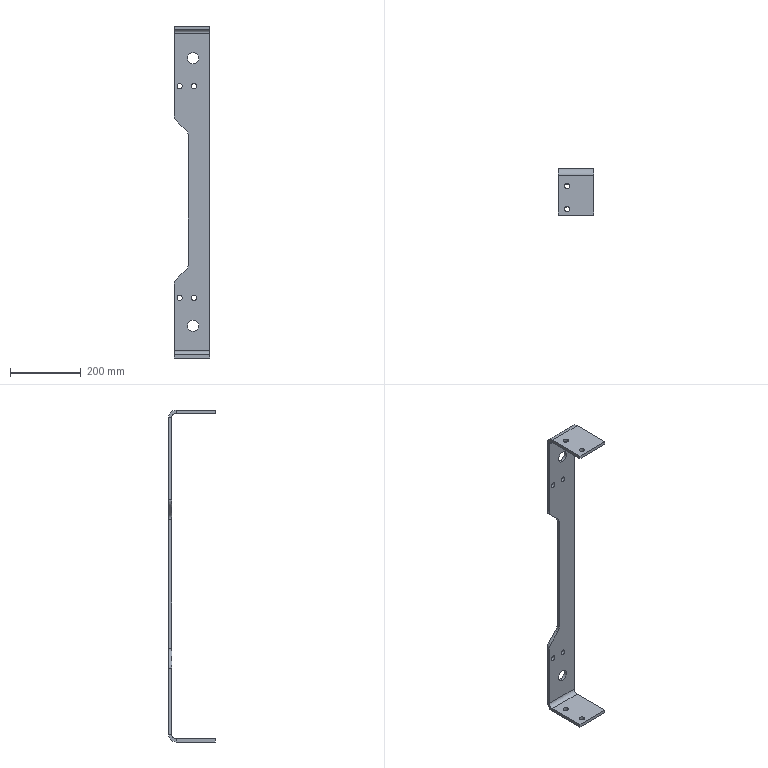Part | SolidWorks | features ICE 2, Fillet 1, FlatPattern 1, SMBaseFlange 1, SheetMetal 1 | 1 solid | 50 faces | box 100 x 132 x 940 mm | volume 876071 mm3 | cylinder 28 | plane 22 | commonest cylinder face diameters 15 x16 32.2 x4 40 x4 24 x2 42 x2
STEP:
#1=CARTESIAN_POINT('',(32.5,17.,-931.));
#2=VERTEX_POINT('',#1);
#3=CARTESIAN_POINT('',(17.5,17.,-931.));
#4=VERTEX_POINT('',#3);
#5=CARTESIAN_POINT('',(25.,17.,-931.));
#6=DIRECTION('',(0.,0.,-1.));
#7=DIRECTION('',(-1.,0.,0.));
#8=AXIS2_PLACEMENT_3D('',#5,#6,#7);
#9=CIRCLE('',#8,7.5);
#10=EDGE_CURVE('',#2,#4,#9,.T.);
#11=ORIENTED_EDGE('',*,*,#10,.F.);
#12=CARTESIAN_POINT('',(32.5,17.,-940.));
#13=VERTEX_POINT('',#12);
#14=CARTESIAN_POINT('',(32.5,17.,0.));
#15=DIRECTION('',(0.,0.,-1.));
#16=VECTOR('',#15,1000.);
#17=LINE('',#14,#16);
#18=EDGE_CURVE('',#2,#13,#17,.T.);
#19=ORIENTED_EDGE('',*,*,#18,.T.);
#20=CARTESIAN_POINT('',(17.5,17.,-940.));
#21=VERTEX_POINT('',#20);
#22=CARTESIAN_POINT('',(25.,17.,-940.));
#23=DIRECTION('',(0.,0.,-1.));
#24=DIRECTION('',(-1.,0.,0.));
#25=AXIS2_PLACEMENT_3D('',#22,#23,#24);
#26=CIRCLE('',#25,7.5);
#27=EDGE_CURVE('',#13,#21,#26,.T.);
#28=ORIENTED_EDGE('',*,*,#27,.T.);
#29=CARTESIAN_POINT('',(17.5,17.,0.));
#30=DIRECTION('',(0.,0.,-1.));
#31=VECTOR('',#30,1000.);
#32=LINE('',#29,#31);
#33=EDGE_CURVE('',#4,#21,#32,.T.);
#34=ORIENTED_EDGE('',*,*,#33,.F.);
#35=EDGE_LOOP('',(#11,#19,#28,#34));
#36=FACE_OUTER_BOUND('',#35,.T.);
#37=CARTESIAN_POINT('',(25.,17.,0.));
#38=DIRECTION('',(0.,0.,-1.));
#39=DIRECTION('',(-1.,0.,0.));
#40=AXIS2_PLACEMENT_3D('',#37,#38,#39);
#41=CYLINDRICAL_SURFACE('',#40,7.5);
#42=ADVANCED_FACE('',(#36),#41,.F.);
#43=CARTESIAN_POINT('',(32.5,82.,-931.));
#44=VERTEX_POINT('',#43);
#45=CARTESIAN_POINT('',(17.5,82.,-931.));
#46=VERTEX_POINT('',#45);
#47=CARTESIAN_POINT('',(25.,82.,-931.));
#48=DIRECTION('',(0.,0.,-1.));
#49=DIRECTION('',(-1.,0.,0.));
#50=AXIS2_PLACEMENT_3D('',#47,#48,#49);
#51=CIRCLE('',#50,7.5);
#52=EDGE_CURVE('',#44,#46,#51,.T.);
#53=ORIENTED_EDGE('',*,*,#52,.F.);
#54=CARTESIAN_POINT('',(32.5,82.,-940.));
#55=VERTEX_POINT('',#54);
#56=CARTESIAN_POINT('',(32.5,82.,0.));
#57=DIRECTION('',(0.,0.,-1.));
#58=VECTOR('',#57,1000.);
#59=LINE('',#56,#58);
#60=EDGE_CURVE('',#44,#55,#59,.T.);
#61=ORIENTED_EDGE('',*,*,#60,.T.);
#62=CARTESIAN_POINT('',(17.5,82.,-940.));
#63=VERTEX_POINT('',#62);
#64=CARTESIAN_POINT('',(25.,82.,-940.));
#65=DIRECTION('',(0.,0.,-1.));
#66=DIRECTION('',(-1.,0.,0.));
#67=AXIS2_PLACEMENT_3D('',#64,#65,#66);
#68=CIRCLE('',#67,7.5);
#69=EDGE_CURVE('',#55,#63,#68,.T.);
#70=ORIENTED_EDGE('',*,*,#69,.T.);
#71=CARTESIAN_POINT('',(17.5,82.,0.));
#72=DIRECTION('',(0.,0.,-1.));
#73=VECTOR('',#72,1000.);
#74=LINE('',#71,#73);
#75=EDGE_CURVE('',#46,#63,#74,.T.);
#76=ORIENTED_EDGE('',*,*,#75,.F.);
#77=EDGE_LOOP('',(#53,#61,#70,#76));
#78=FACE_OUTER_BOUND('',#77,.T.);
#79=CARTESIAN_POINT('',(25.,82.,0.));
#80=DIRECTION('',(0.,0.,-1.));
#81=DIRECTION('',(-1.,0.,0.));
#82=AXIS2_PLACEMENT_3D('',#79,#80,#81);
#83=CYLINDRICAL_SURFACE('',#82,7.5);
#84=ADVANCED_FACE('',(#78),#83,.F.);
#85=CARTESIAN_POINT('',(32.5,17.,0.));
#86=VERTEX_POINT('',#85);
#87=CARTESIAN_POINT('',(17.5,17.,0.));
#88=VERTEX_POINT('',#87);
#89=CARTESIAN_POINT('',(25.,17.,0.));
#90=DIRECTION('',(0.,0.,-1.));
#91=DIRECTION('',(-1.,0.,0.));
#92=AXIS2_PLACEMENT_3D('',#89,#90,#91);
#93=CIRCLE('',#92,7.5);
#94=EDGE_CURVE('',#86,#88,#93,.T.);
#95=ORIENTED_EDGE('',*,*,#94,.F.);
#96=CARTESIAN_POINT('',(32.5,17.,-9.));
#97=VERTEX_POINT('',#96);
#98=CARTESIAN_POINT('',(32.5,17.,0.));
#99=DIRECTION('',(0.,0.,-1.));
#100=VECTOR('',#99,1000.);
#101=LINE('',#98,#100);
#102=EDGE_CURVE('',#86,#97,#101,.T.);
#103=ORIENTED_EDGE('',*,*,#102,.T.);
#104=CARTESIAN_POINT('',(17.5,17.,-9.));
#105=VERTEX_POINT('',#104);
#106=CARTESIAN_POINT('',(25.,17.,-9.));
#107=DIRECTION('',(0.,0.,1.));
#108=DIRECTION('',(1.,0.,0.));
#109=AXIS2_PLACEMENT_3D('',#106,#107,#108);
#110=CIRCLE('',#109,7.5);
#111=EDGE_CURVE('',#105,#97,#110,.T.);
#112=ORIENTED_EDGE('',*,*,#111,.F.);
#113=CARTESIAN_POINT('',(17.5,17.,0.));
#114=DIRECTION('',(0.,0.,-1.));
#115=VECTOR('',#114,1000.);
#116=LINE('',#113,#115);
#117=EDGE_CURVE('',#88,#105,#116,.T.);
#118=ORIENTED_EDGE('',*,*,#117,.F.);
#119=EDGE_LOOP('',(#95,#103,#112,#118));
#120=FACE_OUTER_BOUND('',#119,.T.);
#121=CARTESIAN_POINT('',(25.,17.,0.));
#122=DIRECTION('',(0.,0.,-1.));
#123=DIRECTION('',(-1.,0.,0.));
#124=AXIS2_PLACEMENT_3D('',#121,#122,#123);
#125=CYLINDRICAL_SURFACE('',#124,7.5);
#126=ADVANCED_FACE('',(#120),#125,.F.);
#127=CARTESIAN_POINT('',(32.5,82.,0.));
#128=VERTEX_POINT('',#127);
#129=CARTESIAN_POINT('',(17.5,82.,0.));
#130=VERTEX_POINT('',#129);
#131=CARTESIAN_POINT('',(25.,82.,0.));
#132=DIRECTION('',(0.,0.,-1.));
#133=DIRECTION('',(-1.,0.,0.));
#134=AXIS2_PLACEMENT_3D('',#131,#132,#133);
#135=CIRCLE('',#134,7.5);
#136=EDGE_CURVE('',#128,#130,#135,.T.);
#137=ORIENTED_EDGE('',*,*,#136,.F.);
#138=CARTESIAN_POINT('',(32.5,82.,-9.));
#139=VERTEX_POINT('',#138);
#140=CARTESIAN_POINT('',(32.5,82.,0.));
#141=DIRECTION('',(0.,0.,-1.));
#142=VECTOR('',#141,1000.);
#143=LINE('',#140,#142);
#144=EDGE_CURVE('',#128,#139,#143,.T.);
#145=ORIENTED_EDGE('',*,*,#144,.T.);
#146=CARTESIAN_POINT('',(17.5,82.,-9.));
#147=VERTEX_POINT('',#146);
#148=CARTESIAN_POINT('',(25.,82.,-9.));
#149=DIRECTION('',(0.,0.,1.));
#150=DIRECTION('',(1.,0.,0.));
#151=AXIS2_PLACEMENT_3D('',#148,#149,#150);
#152=CIRCLE('',#151,7.5);
#153=EDGE_CURVE('',#147,#139,#152,.T.);
#154=ORIENTED_EDGE('',*,*,#153,.F.);
#155=CARTESIAN_POINT('',(17.5,82.,0.));
#156=DIRECTION('',(0.,0.,-1.));
#157=VECTOR('',#156,1000.);
#158=LINE('',#155,#157);
#159=EDGE_CURVE('',#130,#147,#158,.T.);
#160=ORIENTED_EDGE('',*,*,#159,.F.);
#161=EDGE_LOOP('',(#137,#145,#154,#160));
#162=FACE_OUTER_BOUND('',#161,.T.);
#163=CARTESIAN_POINT('',(25.,82.,0.));
#164=DIRECTION('',(0.,0.,-1.));
#165=DIRECTION('',(-1.,0.,0.));
#166=AXIS2_PLACEMENT_3D('',#163,#164,#165);
#167=CYLINDRICAL_SURFACE('',#166,7.5);
#168=ADVANCED_FACE('',(#162),#167,.F.);
#169=CARTESIAN_POINT('',(55.2,123.,-777.5));
#170=VERTEX_POINT('',#169);
#171=CARTESIAN_POINT('',(55.2,123.,-762.5));
#172=VERTEX_POINT('',#171);
#173=CARTESIAN_POINT('',(55.2,123.,-770.));
#174=DIRECTION('',(0.,1.,0.));
#175=DIRECTION('',(0.,0.,1.));
#176=AXIS2_PLACEMENT_3D('',#173,#174,#175);
#177=CIRCLE('',#176,7.5);
#178=EDGE_CURVE('',#170,#172,#177,.T.);
#179=ORIENTED_EDGE('',*,*,#178,.F.);
#180=CARTESIAN_POINT('',(55.2,132.,-777.5));
#181=VERTEX_POINT('',#180);
#182=CARTESIAN_POINT('',(55.2,132.,-777.5));
#183=DIRECTION('',(0.,1.,0.));
#184=VECTOR('',#183,1000.);
#185=LINE('',#182,#184);
#186=EDGE_CURVE('',#170,#181,#185,.T.);
#187=ORIENTED_EDGE('',*,*,#186,.T.);
#188=CARTESIAN_POINT('',(55.2,132.,-762.5));
#189=VERTEX_POINT('',#188);
#190=CARTESIAN_POINT('',(55.2,132.,-770.));
#191=DIRECTION('',(0.,1.,0.));
#192=DIRECTION('',(0.,0.,1.));
#193=AXIS2_PLACEMENT_3D('',#190,#191,#192);
#194=CIRCLE('',#193,7.5);
#195=EDGE_CURVE('',#181,#189,#194,.T.);
#196=ORIENTED_EDGE('',*,*,#195,.T.);
#197=CARTESIAN_POINT('',(55.2,132.,-762.5));
#198=DIRECTION('',(0.,1.,0.));
#199=VECTOR('',#198,1000.);
#200=LINE('',#197,#199);
#201=EDGE_CURVE('',#172,#189,#200,.T.);
#202=ORIENTED_EDGE('',*,*,#201,.F.);
#203=EDGE_LOOP('',(#179,#187,#196,#202));
#204=FACE_OUTER_BOUND('',#203,.T.);
#205=CARTESIAN_POINT('',(55.2,132.,-770.));
#206=DIRECTION('',(0.,1.,0.));
#207=DIRECTION('',(0.,0.,1.));
#208=AXIS2_PLACEMENT_3D('',#205,#206,#207);
#209=CYLINDRICAL_SURFACE('',#208,7.5);
#210=ADVANCED_FACE('',(#204),#209,.F.);
#211=CARTESIAN_POINT('',(15.2,123.,-177.5));
#212=VERTEX_POINT('',#211);
#213=CARTESIAN_POINT('',(15.2,123.,-162.5));
#214=VERTEX_POINT('',#213);
#215=CARTESIAN_POINT('',(15.2,123.,-170.));
#216=DIRECTION('',(0.,1.,0.));
#217=DIRECTION('',(0.,0.,1.));
#218=AXIS2_PLACEMENT_3D('',#215,#216,#217);
#219=CIRCLE('',#218,7.5);
#220=EDGE_CURVE('',#212,#214,#219,.T.);
#221=ORIENTED_EDGE('',*,*,#220,.F.);
#222=CARTESIAN_POINT('',(15.2,132.,-177.5));
#223=VERTEX_POINT('',#222);
#224=CARTESIAN_POINT('',(15.2,132.,-177.5));
#225=DIRECTION('',(0.,1.,0.));
#226=VECTOR('',#225,1000.);
#227=LINE('',#224,#226);
#228=EDGE_CURVE('',#212,#223,#227,.T.);
#229=ORIENTED_EDGE('',*,*,#228,.T.);
#230=CARTESIAN_POINT('',(15.2,132.,-162.5));
#231=VERTEX_POINT('',#230);
#232=CARTESIAN_POINT('',(15.2,132.,-170.));
#233=DIRECTION('',(0.,1.,0.));
#234=DIRECTION('',(0.,0.,1.));
#235=AXIS2_PLACEMENT_3D('',#232,#233,#234);
#236=CIRCLE('',#235,7.5);
#237=EDGE_CURVE('',#223,#231,#236,.T.);
#238=ORIENTED_EDGE('',*,*,#237,.T.);
#239=CARTESIAN_POINT('',(15.2,132.,-162.5));
#240=DIRECTION('',(0.,1.,0.));
#241=VECTOR('',#240,1000.);
#242=LINE('',#239,#241);
#243=EDGE_CURVE('',#214,#231,#242,.T.);
#244=ORIENTED_EDGE('',*,*,#243,.F.);
#245=EDGE_LOOP('',(#221,#229,#238,#244));
#246=FACE_OUTER_BOUND('',#245,.T.);
#247=CARTESIAN_POINT('',(15.2,132.,-170.));
#248=DIRECTION('',(0.,1.,0.));
#249=DIRECTION('',(0.,0.,1.));
#250=AXIS2_PLACEMENT_3D('',#247,#248,#249);
#251=CYLINDRICAL_SURFACE('',#250,7.5);
#252=ADVANCED_FACE('',(#246),#251,.F.);
#253=CARTESIAN_POINT('',(53.,123.,-865.1));
#254=VERTEX_POINT('',#253);
#255=CARTESIAN_POINT('',(53.,123.,-832.9));
#256=VERTEX_POINT('',#255);
#257=CARTESIAN_POINT('',(53.,123.,-849.));
#258=DIRECTION('',(0.,1.,0.));
#259=DIRECTION('',(0.,0.,1.));
#260=AXIS2_PLACEMENT_3D('',#257,#258,#259);
#261=CIRCLE('',#260,16.1);
#262=EDGE_CURVE('',#254,#256,#261,.T.);
#263=ORIENTED_EDGE('',*,*,#262,.F.);
#264=CARTESIAN_POINT('',(53.,132.,-865.1));
#265=VERTEX_POINT('',#264);
#266=CARTESIAN_POINT('',(53.,132.,-865.1));
#267=DIRECTION('',(0.,1.,0.));
#268=VECTOR('',#267,1000.);
#269=LINE('',#266,#268);
#270=EDGE_CURVE('',#254,#265,#269,.T.);
#271=ORIENTED_EDGE('',*,*,#270,.T.);
#272=CARTESIAN_POINT('',(53.,132.,-832.9));
#273=VERTEX_POINT('',#272);
#274=CARTESIAN_POINT('',(53.,132.,-849.));
#275=DIRECTION('',(0.,1.,0.));
#276=DIRECTION('',(0.,0.,1.));
#277=AXIS2_PLACEMENT_3D('',#274,#275,#276);
#278=CIRCLE('',#277,16.1);
#279=EDGE_CURVE('',#265,#273,#278,.T.);
#280=ORIENTED_EDGE('',*,*,#279,.T.);
#281=CARTESIAN_POINT('',(53.,132.,-832.9));
#282=DIRECTION('',(0.,1.,0.));
#283=VECTOR('',#282,1000.);
#284=LINE('',#281,#283);
#285=EDGE_CURVE('',#256,#273,#284,.T.);
#286=ORIENTED_EDGE('',*,*,#285,.F.);
#287=EDGE_LOOP('',(#263,#271,#280,#286));
#288=FACE_OUTER_BOUND('',#287,.T.);
#289=CARTESIAN_POINT('',(53.,132.,-849.));
#290=DIRECTION('',(0.,1.,0.));
#291=DIRECTION('',(0.,0.,1.));
#292=AXIS2_PLACEMENT_3D('',#289,#290,#291);
#293=CYLINDRICAL_SURFACE('',#292,16.1);
#294=ADVANCED_FACE('',(#288),#293,.F.);
#295=CARTESIAN_POINT('',(15.2,123.,-777.5));
#296=VERTEX_POINT('',#295);
#297=CARTESIAN_POINT('',(15.2,123.,-762.5));
#298=VERTEX_POINT('',#297);
#299=CARTESIAN_POINT('',(15.2,123.,-770.));
#300=DIRECTION('',(0.,1.,0.));
#301=DIRECTION('',(0.,0.,1.));
#302=AXIS2_PLACEMENT_3D('',#299,#300,#301);
#303=CIRCLE('',#302,7.5);
#304=EDGE_CURVE('',#296,#298,#303,.T.);
#305=ORIENTED_EDGE('',*,*,#304,.F.);
#306=CARTESIAN_POINT('',(15.2,132.,-777.5));
#307=VERTEX_POINT('',#306);
#308=CARTESIAN_POINT('',(15.2,132.,-777.5));
#309=DIRECTION('',(0.,1.,0.));
#310=VECTOR('',#309,1000.);
#311=LINE('',#308,#310);
#312=EDGE_CURVE('',#296,#307,#311,.T.);
#313=ORIENTED_EDGE('',*,*,#312,.T.);
#314=CARTESIAN_POINT('',(15.2,132.,-762.5));
#315=VERTEX_POINT('',#314);
#316=CARTESIAN_POINT('',(15.2,132.,-770.));
#317=DIRECTION('',(0.,1.,0.));
#318=DIRECTION('',(0.,0.,1.));
#319=AXIS2_PLACEMENT_3D('',#316,#317,#318);
#320=CIRCLE('',#319,7.5);
#321=EDGE_CURVE('',#307,#315,#320,.T.);
#322=ORIENTED_EDGE('',*,*,#321,.T.);
#323=CARTESIAN_POINT('',(15.2,132.,-762.5));
#324=DIRECTION('',(0.,1.,0.));
#325=VECTOR('',#324,1000.);
#326=LINE('',#323,#325);
#327=EDGE_CURVE('',#298,#315,#326,.T.);
#328=ORIENTED_EDGE('',*,*,#327,.F.);
#329=EDGE_LOOP('',(#305,#313,#322,#328));
#330=FACE_OUTER_BOUND('',#329,.T.);
#331=CARTESIAN_POINT('',(15.2,132.,-770.));
#332=DIRECTION('',(0.,1.,0.));
#333=DIRECTION('',(0.,0.,1.));
#334=AXIS2_PLACEMENT_3D('',#331,#332,#333);
#335=CYLINDRICAL_SURFACE('',#334,7.5);
#336=ADVANCED_FACE('',(#330),#335,.F.);
#337=CARTESIAN_POINT('',(53.,123.,-107.1));
#338=VERTEX_POINT('',#337);
#339=CARTESIAN_POINT('',(53.,123.,-74.9));
#340=VERTEX_POINT('',#339);
#341=CARTESIAN_POINT('',(53.,123.,-91.));
#342=DIRECTION('',(0.,1.,0.));
#343=DIRECTION('',(0.,0.,1.));
#344=AXIS2_PLACEMENT_3D('',#341,#342,#343);
#345=CIRCLE('',#344,16.1);
#346=EDGE_CURVE('',#338,#340,#345,.T.);
#347=ORIENTED_EDGE('',*,*,#346,.F.);
#348=CARTESIAN_POINT('',(53.,132.,-107.1));
#349=VERTEX_POINT('',#348);
#350=CARTESIAN_POINT('',(53.,132.,-107.1));
#351=DIRECTION('',(0.,1.,0.));
#352=VECTOR('',#351,1000.);
#353=LINE('',#350,#352);
#354=EDGE_CURVE('',#338,#349,#353,.T.);
#355=ORIENTED_EDGE('',*,*,#354,.T.);
#356=CARTESIAN_POINT('',(53.,132.,-74.9));
#357=VERTEX_POINT('',#356);
#358=CARTESIAN_POINT('',(53.,132.,-91.));
#359=DIRECTION('',(0.,1.,0.));
#360=DIRECTION('',(0.,0.,1.));
#361=AXIS2_PLACEMENT_3D('',#358,#359,#360);
#362=CIRCLE('',#361,16.1);
#363=EDGE_CURVE('',#349,#357,#362,.T.);
#364=ORIENTED_EDGE('',*,*,#363,.T.);
#365=CARTESIAN_POINT('',(53.,132.,-74.9));
#366=DIRECTION('',(0.,1.,0.));
#367=VECTOR('',#366,1000.);
#368=LINE('',#365,#367);
#369=EDGE_CURVE('',#340,#357,#368,.T.);
#370=ORIENTED_EDGE('',*,*,#369,.F.);
#371=EDGE_LOOP('',(#347,#355,#364,#370));
#372=FACE_OUTER_BOUND('',#371,.T.);
#373=CARTESIAN_POINT('',(53.,132.,-91.));
#374=DIRECTION('',(0.,1.,0.));
#375=DIRECTION('',(0.,0.,1.));
#376=AXIS2_PLACEMENT_3D('',#373,#374,#375);
#377=CYLINDRICAL_SURFACE('',#376,16.1);
#378=ADVANCED_FACE('',(#372),#377,.F.);
#379=CARTESIAN_POINT('',(55.2,123.,-177.5));
#380=VERTEX_POINT('',#379);
#381=CARTESIAN_POINT('',(55.2,123.,-162.5));
#382=VERTEX_POINT('',#381);
#383=CARTESIAN_POINT('',(55.2,123.,-170.));
#384=DIRECTION('',(0.,1.,0.));
#385=DIRECTION('',(0.,0.,1.));
#386=AXIS2_PLACEMENT_3D('',#383,#384,#385);
#387=CIRCLE('',#386,7.5);
#388=EDGE_CURVE('',#380,#382,#387,.T.);
#389=ORIENTED_EDGE('',*,*,#388,.F.);
#390=CARTESIAN_POINT('',(55.2,132.,-177.5));
#391=VERTEX_POINT('',#390);
#392=CARTESIAN_POINT('',(55.2,132.,-177.5));
#393=DIRECTION('',(0.,1.,0.));
#394=VECTOR('',#393,1000.);
#395=LINE('',#392,#394);
#396=EDGE_CURVE('',#380,#391,#395,.T.);
#397=ORIENTED_EDGE('',*,*,#396,.T.);
#398=CARTESIAN_POINT('',(55.2,132.,-162.5));
#399=VERTEX_POINT('',#398);
#400=CARTESIAN_POINT('',(55.2,132.,-170.));
#401=DIRECTION('',(0.,1.,0.));
#402=DIRECTION('',(0.,0.,1.));
#403=AXIS2_PLACEMENT_3D('',#400,#401,#402);
#404=CIRCLE('',#403,7.5);
#405=EDGE_CURVE('',#391,#399,#404,.T.);
#406=ORIENTED_EDGE('',*,*,#405,.T.);
#407=CARTESIAN_POINT('',(55.2,132.,-162.5));
#408=DIRECTION('',(0.,1.,0.));
#409=VECTOR('',#408,1000.);
#410=LINE('',#407,#409);
#411=EDGE_CURVE('',#382,#399,#410,.T.);
#412=ORIENTED_EDGE('',*,*,#411,.F.);
#413=EDGE_LOOP('',(#389,#397,#406,#412));
#414=FACE_OUTER_BOUND('',#413,.T.);
#415=CARTESIAN_POINT('',(55.2,132.,-170.));
#416=DIRECTION('',(0.,1.,0.));
#417=DIRECTION('',(0.,0.,1.));
#418=AXIS2_PLACEMENT_3D('',#415,#416,#417);
#419=CYLINDRICAL_SURFACE('',#418,7.5);
#420=ADVANCED_FACE('',(#414),#419,.F.);
#421=CARTESIAN_POINT('',(0.,132.,-21.));
#422=VERTEX_POINT('',#421);
#423=CARTESIAN_POINT('',(0.,132.,-254.216));
#424=VERTEX_POINT('',#423);
#425=CARTESIAN_POINT('',(0.,132.,0.));
#426=DIRECTION('',(0.,0.,-1.));
#427=VECTOR('',#426,1000.);
#428=LINE('',#425,#427);
#429=EDGE_CURVE('',#422,#424,#428,.T.);
#430=ORIENTED_EDGE('',*,*,#429,.T.);
#431=CARTESIAN_POINT('',(0.,123.,-254.216));
#432=VERTEX_POINT('',#431);
#433=CARTESIAN_POINT('',(0.,111.,-254.216));
#434=DIRECTION('',(0.,-1.,0.));
#435=VECTOR('',#434,1000.);
#436=LINE('',#433,#435);
#437=EDGE_CURVE('',#424,#432,#436,.T.);
#438=ORIENTED_EDGE('',*,*,#437,.T.);
#439=CARTESIAN_POINT('',(0.,123.,-21.));
#440=VERTEX_POINT('',#439);
#441=CARTESIAN_POINT('',(0.,123.,0.));
#442=DIRECTION('',(0.,0.,-1.));
#443=VECTOR('',#442,1000.);
#444=LINE('',#441,#443);
#445=EDGE_CURVE('',#440,#432,#444,.T.);
#446=ORIENTED_EDGE('',*,*,#445,.F.);
#447=CARTESIAN_POINT('',(0.,123.,-21.));
#448=DIRECTION('',(0.,1.,0.));
#449=VECTOR('',#448,1000.);
#450=LINE('',#447,#449);
#451=EDGE_CURVE('',#440,#422,#450,.T.);
#452=ORIENTED_EDGE('',*,*,#451,.T.);
#453=EDGE_LOOP('',(#430,#438,#446,#452));
#454=FACE_OUTER_BOUND('',#453,.T.);
#455=CARTESIAN_POINT('',(0.,111.,-931.));
#456=DIRECTION('',(-1.,0.,0.));
#457=DIRECTION('',(0.,0.,1.));
#458=AXIS2_PLACEMENT_3D('',#455,#456,#457);
#459=PLANE('',#458);
#460=ADVANCED_FACE('',(#454),#459,.T.);
#461=CARTESIAN_POINT('',(0.,123.,-730.784));
#462=VERTEX_POINT('',#461);
#463=CARTESIAN_POINT('',(0.,123.,-919.));
#464=VERTEX_POINT('',#463);
#465=CARTESIAN_POINT('',(0.,123.,0.));
#466=DIRECTION('',(0.,0.,-1.));
#467=VECTOR('',#466,1000.);
#468=LINE('',#465,#467);
#469=EDGE_CURVE('',#462,#464,#468,.T.);
#470=ORIENTED_EDGE('',*,*,#469,.F.);
#471=CARTESIAN_POINT('',(0.,132.,-730.784));
#472=VERTEX_POINT('',#471);
#473=CARTESIAN_POINT('',(0.,111.,-730.784));
#474=DIRECTION('',(0.,1.,0.));
#475=VECTOR('',#474,1000.);
#476=LINE('',#473,#475);
#477=EDGE_CURVE('',#462,#472,#476,.T.);
#478=ORIENTED_EDGE('',*,*,#477,.T.);
#479=CARTESIAN_POINT('',(0.,132.,-919.));
#480=VERTEX_POINT('',#479);
#481=CARTESIAN_POINT('',(0.,132.,0.));
#482=DIRECTION('',(0.,0.,-1.));
#483=VECTOR('',#482,1000.);
#484=LINE('',#481,#483);
#485=EDGE_CURVE('',#472,#480,#484,.T.);
#486=ORIENTED_EDGE('',*,*,#485,.T.);
#487=CARTESIAN_POINT('',(0.,132.,-919.));
#488=DIRECTION('',(0.,-1.,0.));
#489=VECTOR('',#488,1000.);
#490=LINE('',#487,#489);
#491=EDGE_CURVE('',#480,#464,#490,.T.);
#492=ORIENTED_EDGE('',*,*,#491,.T.);
#493=EDGE_LOOP('',(#470,#478,#486,#492));
#494=FACE_OUTER_BOUND('',#493,.T.);
#495=CARTESIAN_POINT('',(0.,111.,-931.));
#496=DIRECTION('',(-1.,0.,0.));
#497=DIRECTION('',(0.,0.,1.));
#498=AXIS2_PLACEMENT_3D('',#495,#496,#497);
#499=PLANE('',#498);
#500=ADVANCED_FACE('',(#494),#499,.T.);
#501=CARTESIAN_POINT('',(100.,132.,-21.));
#502=VERTEX_POINT('',#501);
#503=CARTESIAN_POINT('',(100.,123.,-21.));
#504=VERTEX_POINT('',#503);
#505=CARTESIAN_POINT('',(100.,132.,-21.));
#506=DIRECTION('',(0.,-1.,0.));
#507=VECTOR('',#506,1000.);
#508=LINE('',#505,#507);
#509=EDGE_CURVE('',#502,#504,#508,.T.);
#510=ORIENTED_EDGE('',*,*,#509,.F.);
#511=CARTESIAN_POINT('',(100.,111.,0.));
#512=VERTEX_POINT('',#511);
#513=CARTESIAN_POINT('',(100.,111.,-21.));
#514=DIRECTION('',(-1.,0.,0.));
#515=DIRECTION('',(0.,0.,-1.));
#516=AXIS2_PLACEMENT_3D('',#513,#514,#515);
#517=CIRCLE('',#516,21.);
#518=EDGE_CURVE('',#512,#502,#517,.T.);
#519=ORIENTED_EDGE('',*,*,#518,.F.);
#520=CARTESIAN_POINT('',(100.,111.,-9.));
#521=VERTEX_POINT('',#520);
#522=CARTESIAN_POINT('',(100.,111.,-9.));
#523=DIRECTION('',(0.,0.,1.));
#524=VECTOR('',#523,1000.);
#525=LINE('',#522,#524);
#526=EDGE_CURVE('',#521,#512,#525,.T.);
#527=ORIENTED_EDGE('',*,*,#526,.F.);
#528=CARTESIAN_POINT('',(100.,111.,-21.));
#529=DIRECTION('',(-1.,0.,0.));
#530=DIRECTION('',(0.,0.,-1.));
#531=AXIS2_PLACEMENT_3D('',#528,#529,#530);
#532=CIRCLE('',#531,12.);
#533=EDGE_CURVE('',#521,#504,#532,.T.);
#534=ORIENTED_EDGE('',*,*,#533,.T.);
#535=EDGE_LOOP('',(#510,#519,#527,#534));
#536=FACE_OUTER_BOUND('',#535,.T.);
#537=CARTESIAN_POINT('',(100.,132.,-21.));
#538=DIRECTION('',(1.,0.,0.));
#539=DIRECTION('',(0.,0.,-1.));
#540=AXIS2_PLACEMENT_3D('',#537,#538,#539);
#541=PLANE('',#540);
#542=ADVANCED_FACE('',(#536),#541,.T.);
#543=CARTESIAN_POINT('',(100.,132.,-919.));
#544=VERTEX_POINT('',#543);
#545=CARTESIAN_POINT('',(100.,132.,0.));
#546=DIRECTION('',(0.,0.,-1.));
#547=VECTOR('',#546,1000.);
#548=LINE('',#545,#547);
#549=EDGE_CURVE('',#502,#544,#548,.T.);
#550=ORIENTED_EDGE('',*,*,#549,.F.);
#551=ORIENTED_EDGE('',*,*,#509,.T.);
#552=CARTESIAN_POINT('',(100.,123.,-919.));
#553=VERTEX_POINT('',#552);
#554=CARTESIAN_POINT('',(100.,123.,0.));
#555=DIRECTION('',(0.,0.,-1.));
#556=VECTOR('',#555,1000.);
#557=LINE('',#554,#556);
#558=EDGE_CURVE('',#504,#553,#557,.T.);
#559=ORIENTED_EDGE('',*,*,#558,.T.);
#560=CARTESIAN_POINT('',(100.,123.,-919.));
#561=DIRECTION('',(0.,1.,0.));
#562=VECTOR('',#561,1000.);
#563=LINE('',#560,#562);
#564=EDGE_CURVE('',#553,#544,#563,.T.);
#565=ORIENTED_EDGE('',*,*,#564,.T.);
#566=EDGE_LOOP('',(#550,#551,#559,#565));
#567=FACE_OUTER_BOUND('',#566,.T.);
#568=CARTESIAN_POINT('',(100.,111.,-9.));
#569=DIRECTION('',(1.,0.,0.));
#570=DIRECTION('',(0.,0.,-1.));
#571=AXIS2_PLACEMENT_3D('',#568,#569,#570);
#572=PLANE('',#571);
#573=ADVANCED_FACE('',(#567),#572,.T.);
#574=CARTESIAN_POINT('',(0.,111.,0.));
#575=VERTEX_POINT('',#574);
#576=CARTESIAN_POINT('',(0.,111.,-9.));
#577=VERTEX_POINT('',#576);
#578=CARTESIAN_POINT('',(0.,111.,0.));
#579=DIRECTION('',(0.,0.,-1.));
#580=VECTOR('',#579,1000.);
#581=LINE('',#578,#580);
#582=EDGE_CURVE('',#575,#577,#581,.T.);
#583=ORIENTED_EDGE('',*,*,#582,.F.);
#584=CARTESIAN_POINT('',(0.,111.,-21.));
#585=DIRECTION('',(-1.,0.,0.));
#586=DIRECTION('',(0.,0.,-1.));
#587=AXIS2_PLACEMENT_3D('',#584,#585,#586);
#588=CIRCLE('',#587,21.);
#589=EDGE_CURVE('',#575,#422,#588,.T.);
#590=ORIENTED_EDGE('',*,*,#589,.T.);
#591=ORIENTED_EDGE('',*,*,#451,.F.);
#592=CARTESIAN_POINT('',(0.,111.,-21.));
#593=DIRECTION('',(-1.,0.,0.));
#594=DIRECTION('',(0.,0.,-1.));
#595=AXIS2_PLACEMENT_3D('',#592,#593,#594);
#596=CIRCLE('',#595,12.);
#597=EDGE_CURVE('',#577,#440,#596,.T.);
#598=ORIENTED_EDGE('',*,*,#597,.F.);
#599=EDGE_LOOP('',(#583,#590,#591,#598));
#600=FACE_OUTER_BOUND('',#599,.T.);
#601=CARTESIAN_POINT('',(0.,111.,0.));
#602=DIRECTION('',(-1.,0.,0.));
#603=DIRECTION('',(0.,0.,1.));
#604=AXIS2_PLACEMENT_3D('',#601,#602,#603);
#605=PLANE('',#604);
#606=ADVANCED_FACE('',(#600),#605,.T.);
#607=CARTESIAN_POINT('',(0.,0.,0.));
#608=VERTEX_POINT('',#607);
#609=CARTESIAN_POINT('',(0.,0.,0.));
#610=DIRECTION('',(0.,1.,0.));
#611=VECTOR('',#610,1000.);
#612=LINE('',#609,#611);
#613=EDGE_CURVE('',#608,#575,#612,.T.);
#614=ORIENTED_EDGE('',*,*,#613,.T.);
#615=ORIENTED_EDGE('',*,*,#582,.T.);
#616=CARTESIAN_POINT('',(0.,0.,-9.));
#617=VERTEX_POINT('',#616);
#618=CARTESIAN_POINT('',(0.,0.,-9.));
#619=DIRECTION('',(0.,1.,0.));
#620=VECTOR('',#619,1000.);
#621=LINE('',#618,#620);
#622=EDGE_CURVE('',#617,#577,#621,.T.);
#623=ORIENTED_EDGE('',*,*,#622,.F.);
#624=CARTESIAN_POINT('',(0.,0.,-9.));
#625=DIRECTION('',(0.,0.,1.));
#626=VECTOR('',#625,1000.);
#627=LINE('',#624,#626);
#628=EDGE_CURVE('',#617,#608,#627,.T.);
#629=ORIENTED_EDGE('',*,*,#628,.T.);
#630=EDGE_LOOP('',(#614,#615,#623,#629));
#631=FACE_OUTER_BOUND('',#630,.T.);
#632=CARTESIAN_POINT('',(0.,123.,-21.));
#633=DIRECTION('',(-1.,0.,0.));
#634=DIRECTION('',(0.,0.,1.));
#635=AXIS2_PLACEMENT_3D('',#632,#633,#634);
#636=PLANE('',#635);
#637=ADVANCED_FACE('',(#631),#636,.T.);
#638=CARTESIAN_POINT('',(100.,111.,-940.));
#639=VERTEX_POINT('',#638);
#640=CARTESIAN_POINT('',(100.,111.,-931.));
#641=VERTEX_POINT('',#640);
#642=CARTESIAN_POINT('',(100.,111.,-940.));
#643=DIRECTION('',(0.,0.,1.));
#644=VECTOR('',#643,1000.);
#645=LINE('',#642,#644);
#646=EDGE_CURVE('',#639,#641,#645,.T.);
#647=ORIENTED_EDGE('',*,*,#646,.F.);
#648=CARTESIAN_POINT('',(100.,111.,-919.));
#649=DIRECTION('',(-1.,0.,0.));
#650=DIRECTION('',(0.,0.,-1.));
#651=AXIS2_PLACEMENT_3D('',#648,#649,#650);
#652=CIRCLE('',#651,21.);
#653=EDGE_CURVE('',#544,#639,#652,.T.);
#654=ORIENTED_EDGE('',*,*,#653,.F.);
#655=ORIENTED_EDGE('',*,*,#564,.F.);
#656=CARTESIAN_POINT('',(100.,111.,-919.));
#657=DIRECTION('',(-1.,0.,0.));
#658=DIRECTION('',(0.,0.,-1.));
#659=AXIS2_PLACEMENT_3D('',#656,#657,#658);
#660=CIRCLE('',#659,12.);
#661=EDGE_CURVE('',#553,#641,#660,.T.);
#662=ORIENTED_EDGE('',*,*,#661,.T.);
#663=EDGE_LOOP('',(#647,#654,#655,#662));
#664=FACE_OUTER_BOUND('',#663,.T.);
#665=CARTESIAN_POINT('',(100.,111.,-940.));
#666=DIRECTION('',(1.,0.,0.));
#667=DIRECTION('',(0.,0.,-1.));
#668=AXIS2_PLACEMENT_3D('',#665,#666,#667);
#669=PLANE('',#668);
#670=ADVANCED_FACE('',(#664),#669,.T.);
#671=CARTESIAN_POINT('',(100.,0.,-940.));
#672=VERTEX_POINT('',#671);
#673=CARTESIAN_POINT('',(100.,132.,-940.));
#674=DIRECTION('',(0.,-1.,0.));
#675=VECTOR('',#674,1000.);
#676=LINE('',#673,#675);
#677=EDGE_CURVE('',#639,#672,#676,.T.);
#678=ORIENTED_EDGE('',*,*,#677,.F.);
#679=ORIENTED_EDGE('',*,*,#646,.T.);
#680=CARTESIAN_POINT('',(100.,0.,-931.));
#681=VERTEX_POINT('',#680);
#682=CARTESIAN_POINT('',(100.,132.,-931.));
#683=DIRECTION('',(0.,-1.,0.));
#684=VECTOR('',#683,1000.);
#685=LINE('',#682,#684);
#686=EDGE_CURVE('',#641,#681,#685,.T.);
#687=ORIENTED_EDGE('',*,*,#686,.T.);
#688=CARTESIAN_POINT('',(100.,0.,-940.));
#689=DIRECTION('',(0.,0.,1.));
#690=VECTOR('',#689,1000.);
#691=LINE('',#688,#690);
#692=EDGE_CURVE('',#672,#681,#691,.T.);
#693=ORIENTED_EDGE('',*,*,#692,.F.);
#694=EDGE_LOOP('',(#678,#679,#687,#693));
#695=FACE_OUTER_BOUND('',#694,.T.);
#696=CARTESIAN_POINT('',(100.,123.,-919.));
#697=DIRECTION('',(1.,0.,0.));
#698=DIRECTION('',(0.,0.,-1.));
#699=AXIS2_PLACEMENT_3D('',#696,#697,#698);
#700=PLANE('',#699);
#701=ADVANCED_FACE('',(#695),#700,.T.);
#702=ORIENTED_EDGE('',*,*,#491,.F.);
#703=CARTESIAN_POINT('',(0.,111.,-940.));
#704=VERTEX_POINT('',#703);
#705=CARTESIAN_POINT('',(0.,111.,-919.));
#706=DIRECTION('',(-1.,0.,0.));
#707=DIRECTION('',(0.,0.,-1.));
#708=AXIS2_PLACEMENT_3D('',#705,#706,#707);
#709=CIRCLE('',#708,21.);
#710=EDGE_CURVE('',#480,#704,#709,.T.);
#711=ORIENTED_EDGE('',*,*,#710,.T.);
#712=CARTESIAN_POINT('',(0.,111.,-931.));
#713=VERTEX_POINT('',#712);
#714=CARTESIAN_POINT('',(0.,111.,-931.));
#715=DIRECTION('',(0.,0.,-1.));
#716=VECTOR('',#715,1000.);
#717=LINE('',#714,#716);
#718=EDGE_CURVE('',#713,#704,#717,.T.);
#719=ORIENTED_EDGE('',*,*,#718,.F.);
#720=CARTESIAN_POINT('',(0.,111.,-919.));
#721=DIRECTION('',(-1.,0.,0.));
#722=DIRECTION('',(0.,0.,-1.));
#723=AXIS2_PLACEMENT_3D('',#720,#721,#722);
#724=CIRCLE('',#723,12.);
#725=EDGE_CURVE('',#464,#713,#724,.T.);
#726=ORIENTED_EDGE('',*,*,#725,.F.);
#727=EDGE_LOOP('',(#702,#711,#719,#726));
#728=FACE_OUTER_BOUND('',#727,.T.);
#729=CARTESIAN_POINT('',(0.,132.,-919.));
#730=DIRECTION('',(-1.,0.,0.));
#731=DIRECTION('',(0.,0.,1.));
#732=AXIS2_PLACEMENT_3D('',#729,#730,#731);
#733=PLANE('',#732);
#734=ADVANCED_FACE('',(#728),#733,.T.);
#735=CARTESIAN_POINT('',(25.,17.,-931.));
#736=DIRECTION('',(0.,0.,-1.));
#737=DIRECTION('',(-1.,0.,0.));
#738=AXIS2_PLACEMENT_3D('',#735,#736,#737);
#739=CIRCLE('',#738,7.5);
#740=EDGE_CURVE('',#4,#2,#739,.T.);
#741=ORIENTED_EDGE('',*,*,#740,.T.);
#742=ORIENTED_EDGE('',*,*,#10,.T.);
#743=EDGE_LOOP('',(#741,#742));
#744=FACE_BOUND('',#743,.T.);
#745=CARTESIAN_POINT('',(25.,82.,-931.));
#746=DIRECTION('',(0.,0.,-1.));
#747=DIRECTION('',(-1.,0.,0.));
#748=AXIS2_PLACEMENT_3D('',#745,#746,#747);
#749=CIRCLE('',#748,7.5);
#750=EDGE_CURVE('',#46,#44,#749,.T.);
#751=ORIENTED_EDGE('',*,*,#750,.T.);
#752=ORIENTED_EDGE('',*,*,#52,.T.);
#753=EDGE_LOOP('',(#751,#752));
#754=FACE_BOUND('',#753,.T.);
#755=CARTESIAN_POINT('',(0.,0.,-931.));
#756=VERTEX_POINT('',#755);
#757=CARTESIAN_POINT('',(0.,132.,-931.));
#758=DIRECTION('',(0.,-1.,0.));
#759=VECTOR('',#758,1000.);
#760=LINE('',#757,#759);
#761=EDGE_CURVE('',#713,#756,#760,.T.);
#762=ORIENTED_EDGE('',*,*,#761,.T.);
#763=CARTESIAN_POINT('',(100.,0.,-931.));
#764=DIRECTION('',(-1.,0.,0.));
#765=VECTOR('',#764,1000.);
#766=LINE('',#763,#765);
#767=EDGE_CURVE('',#681,#756,#766,.T.);
#768=ORIENTED_EDGE('',*,*,#767,.F.);
#769=ORIENTED_EDGE('',*,*,#686,.F.);
#770=CARTESIAN_POINT('',(100.,111.,-931.));
#771=DIRECTION('',(-1.,0.,0.));
#772=VECTOR('',#771,1000.);
#773=LINE('',#770,#772);
#774=EDGE_CURVE('',#641,#713,#773,.T.);
#775=ORIENTED_EDGE('',*,*,#774,.T.);
#776=EDGE_LOOP('',(#762,#768,#769,#775));
#777=FACE_OUTER_BOUND('',#776,.T.);
#778=CARTESIAN_POINT('',(100.,132.,-931.));
#779=DIRECTION('',(0.,0.,-1.));
#780=DIRECTION('',(-1.,0.,0.));
#781=AXIS2_PLACEMENT_3D('',#778,#779,#780);
#782=PLANE('',#781);
#783=ADVANCED_FACE('',(#744,#754,#777),#782,.F.);
#784=CARTESIAN_POINT('',(0.,0.,-940.));
#785=VERTEX_POINT('',#784);
#786=CARTESIAN_POINT('',(0.,0.,-940.));
#787=DIRECTION('',(0.,0.,1.));
#788=VECTOR('',#787,1000.);
#789=LINE('',#786,#788);
#790=EDGE_CURVE('',#785,#756,#789,.T.);
#791=ORIENTED_EDGE('',*,*,#790,.F.);
#792=CARTESIAN_POINT('',(100.,0.,-940.));
#793=DIRECTION('',(-1.,0.,0.));
#794=VECTOR('',#793,1000.);
#795=LINE('',#792,#794);
#796=EDGE_CURVE('',#672,#785,#795,.T.);
#797=ORIENTED_EDGE('',*,*,#796,.F.);
#798=ORIENTED_EDGE('',*,*,#692,.T.);
#799=ORIENTED_EDGE('',*,*,#767,.T.);
#800=EDGE_LOOP('',(#791,#797,#798,#799));
#801=FACE_OUTER_BOUND('',#800,.T.);
#802=CARTESIAN_POINT('',(100.,0.,-940.));
#803=DIRECTION('',(0.,-1.,0.));
#804=DIRECTION('',(0.,0.,-1.));
#805=AXIS2_PLACEMENT_3D('',#802,#803,#804);
#806=PLANE('',#805);
#807=ADVANCED_FACE('',(#801),#806,.T.);
#808=CARTESIAN_POINT('',(25.,17.,-940.));
#809=DIRECTION('',(0.,0.,-1.));
#810=DIRECTION('',(-1.,0.,0.));
#811=AXIS2_PLACEMENT_3D('',#808,#809,#810);
#812=CIRCLE('',#811,7.5);
#813=EDGE_CURVE('',#21,#13,#812,.T.);
#814=ORIENTED_EDGE('',*,*,#813,.F.);
#815=ORIENTED_EDGE('',*,*,#27,.F.);
#816=EDGE_LOOP('',(#814,#815));
#817=FACE_BOUND('',#816,.T.);
#818=CARTESIAN_POINT('',(25.,82.,-940.));
#819=DIRECTION('',(0.,0.,-1.));
#820=DIRECTION('',(-1.,0.,0.));
#821=AXIS2_PLACEMENT_3D('',#818,#819,#820);
#822=CIRCLE('',#821,7.5);
#823=EDGE_CURVE('',#63,#55,#822,.T.);
#824=ORIENTED_EDGE('',*,*,#823,.F.);
#825=ORIENTED_EDGE('',*,*,#69,.F.);
#826=EDGE_LOOP('',(#824,#825));
#827=FACE_BOUND('',#826,.T.);
#828=CARTESIAN_POINT('',(0.,132.,-940.));
#829=DIRECTION('',(0.,-1.,0.));
#830=VECTOR('',#829,1000.);
#831=LINE('',#828,#830);
#832=EDGE_CURVE('',#704,#785,#831,.T.);
#833=ORIENTED_EDGE('',*,*,#832,.F.);
#834=CARTESIAN_POINT('',(100.,111.,-940.));
#835=DIRECTION('',(-1.,0.,0.));
#836=VECTOR('',#835,1000.);
#837=LINE('',#834,#836);
#838=EDGE_CURVE('',#639,#704,#837,.T.);
#839=ORIENTED_EDGE('',*,*,#838,.F.);
#840=ORIENTED_EDGE('',*,*,#677,.T.);
#841=ORIENTED_EDGE('',*,*,#796,.T.);
#842=EDGE_LOOP('',(#833,#839,#840,#841));
#843=FACE_OUTER_BOUND('',#842,.T.);
#844=CARTESIAN_POINT('',(100.,132.,-940.));
#845=DIRECTION('',(0.,0.,-1.));
#846=DIRECTION('',(-1.,0.,0.));
#847=AXIS2_PLACEMENT_3D('',#844,#845,#846);
#848=PLANE('',#847);
#849=ADVANCED_FACE('',(#817,#827,#843),#848,.T.);
#850=ORIENTED_EDGE('',*,*,#710,.F.);
#851=CARTESIAN_POINT('',(100.,132.,-919.));
#852=DIRECTION('',(-1.,0.,0.));
#853=VECTOR('',#852,1000.);
#854=LINE('',#851,#853);
#855=EDGE_CURVE('',#544,#480,#854,.T.);
#856=ORIENTED_EDGE('',*,*,#855,.F.);
#857=ORIENTED_EDGE('',*,*,#653,.T.);
#858=ORIENTED_EDGE('',*,*,#838,.T.);
#859=EDGE_LOOP('',(#850,#856,#857,#858));
#860=FACE_OUTER_BOUND('',#859,.T.);
#861=CARTESIAN_POINT('',(100.,111.,-919.));
#862=DIRECTION('',(-1.,0.,0.));
#863=DIRECTION('',(0.,0.,1.));
#864=AXIS2_PLACEMENT_3D('',#861,#862,#863);
#865=CYLINDRICAL_SURFACE('',#864,21.);
#866=ADVANCED_FACE('',(#860),#865,.T.);
#867=CARTESIAN_POINT('',(55.2,132.,-770.));
#868=DIRECTION('',(0.,1.,0.));
#869=DIRECTION('',(0.,0.,1.));
#870=AXIS2_PLACEMENT_3D('',#867,#868,#869);
#871=CIRCLE('',#870,7.5);
#872=EDGE_CURVE('',#189,#181,#871,.T.);
#873=ORIENTED_EDGE('',*,*,#872,.F.);
#874=ORIENTED_EDGE('',*,*,#195,.F.);
#875=EDGE_LOOP('',(#873,#874));
#876=FACE_BOUND('',#875,.T.);
#877=CARTESIAN_POINT('',(15.2,132.,-170.));
#878=DIRECTION('',(0.,1.,0.));
#879=DIRECTION('',(0.,0.,1.));
#880=AXIS2_PLACEMENT_3D('',#877,#878,#879);
#881=CIRCLE('',#880,7.5);
#882=EDGE_CURVE('',#231,#223,#881,.T.);
#883=ORIENTED_EDGE('',*,*,#882,.F.);
#884=ORIENTED_EDGE('',*,*,#237,.F.);
#885=EDGE_LOOP('',(#883,#884));
#886=FACE_BOUND('',#885,.T.);
#887=CARTESIAN_POINT('',(53.,132.,-849.));
#888=DIRECTION('',(0.,1.,0.));
#889=DIRECTION('',(0.,0.,1.));
#890=AXIS2_PLACEMENT_3D('',#887,#888,#889);
#891=CIRCLE('',#890,16.1);
#892=EDGE_CURVE('',#273,#265,#891,.T.);
#893=ORIENTED_EDGE('',*,*,#892,.F.);
#894=ORIENTED_EDGE('',*,*,#279,.F.);
#895=EDGE_LOOP('',(#893,#894));
#896=FACE_BOUND('',#895,.T.);
#897=CARTESIAN_POINT('',(15.2,132.,-770.));
#898=DIRECTION('',(0.,1.,0.));
#899=DIRECTION('',(0.,0.,1.));
#900=AXIS2_PLACEMENT_3D('',#897,#898,#899);
#901=CIRCLE('',#900,7.5);
#902=EDGE_CURVE('',#315,#307,#901,.T.);
#903=ORIENTED_EDGE('',*,*,#902,.F.);
#904=ORIENTED_EDGE('',*,*,#321,.F.);
#905=EDGE_LOOP('',(#903,#904));
#906=FACE_BOUND('',#905,.T.);
#907=CARTESIAN_POINT('',(53.,132.,-91.));
#908=DIRECTION('',(0.,1.,0.));
#909=DIRECTION('',(0.,0.,1.));
#910=AXIS2_PLACEMENT_3D('',#907,#908,#909);
#911=CIRCLE('',#910,16.1);
#912=EDGE_CURVE('',#357,#349,#911,.T.);
#913=ORIENTED_EDGE('',*,*,#912,.F.);
#914=ORIENTED_EDGE('',*,*,#363,.F.);
#915=EDGE_LOOP('',(#913,#914));
#916=FACE_BOUND('',#915,.T.);
#917=CARTESIAN_POINT('',(55.2,132.,-170.));
#918=DIRECTION('',(0.,1.,0.));
#919=DIRECTION('',(0.,0.,1.));
#920=AXIS2_PLACEMENT_3D('',#917,#918,#919);
#921=CIRCLE('',#920,7.5);
#922=EDGE_CURVE('',#399,#391,#921,.T.);
#923=ORIENTED_EDGE('',*,*,#922,.F.);
#924=ORIENTED_EDGE('',*,*,#405,.F.);
#925=EDGE_LOOP('',(#923,#924));
#926=FACE_BOUND('',#925,.T.);
#927=ORIENTED_EDGE('',*,*,#485,.F.);
#928=CARTESIAN_POINT('',(5.858,132.,-716.642));
#929=VERTEX_POINT('',#928);
#930=CARTESIAN_POINT('',(20.,132.,-730.784));
#931=DIRECTION('',(0.,1.,0.));
#932=DIRECTION('',(0.,0.,1.));
#933=AXIS2_PLACEMENT_3D('',#930,#931,#932);
#934=CIRCLE('',#933,20.);
#935=EDGE_CURVE('',#472,#929,#934,.T.);
#936=ORIENTED_EDGE('',*,*,#935,.T.);
#937=CARTESIAN_POINT('',(34.142,132.,-688.358));
#938=VERTEX_POINT('',#937);
#939=CARTESIAN_POINT('',(34.142,132.,-688.358));
#940=DIRECTION('',(0.7071,0.,0.7071));
#941=VECTOR('',#940,1000.);
#942=LINE('',#939,#941);
#943=EDGE_CURVE('',#929,#938,#942,.T.);
#944=ORIENTED_EDGE('',*,*,#943,.T.);
#945=CARTESIAN_POINT('',(40.,132.,-674.216));
#946=VERTEX_POINT('',#945);
#947=CARTESIAN_POINT('',(20.,132.,-674.216));
#948=DIRECTION('',(0.,-1.,0.));
#949=DIRECTION('',(0.,0.,1.));
#950=AXIS2_PLACEMENT_3D('',#947,#948,#949);
#951=CIRCLE('',#950,20.);
#952=EDGE_CURVE('',#938,#946,#951,.T.);
#953=ORIENTED_EDGE('',*,*,#952,.T.);
#954=CARTESIAN_POINT('',(40.,132.,-310.784));
#955=VERTEX_POINT('',#954);
#956=CARTESIAN_POINT('',(40.,132.,0.));
#957=DIRECTION('',(0.,0.,1.));
#958=VECTOR('',#957,1000.);
#959=LINE('',#956,#958);
#960=EDGE_CURVE('',#946,#955,#959,.T.);
#961=ORIENTED_EDGE('',*,*,#960,.T.);
#962=CARTESIAN_POINT('',(34.142,132.,-296.642));
#963=VERTEX_POINT('',#962);
#964=CARTESIAN_POINT('',(20.,132.,-310.784));
#965=DIRECTION('',(0.,-1.,0.));
#966=DIRECTION('',(0.,0.,1.));
#967=AXIS2_PLACEMENT_3D('',#964,#965,#966);
#968=CIRCLE('',#967,20.);
#969=EDGE_CURVE('',#955,#963,#968,.T.);
#970=ORIENTED_EDGE('',*,*,#969,.T.);
#971=CARTESIAN_POINT('',(5.858,132.,-268.358));
#972=VERTEX_POINT('',#971);
#973=CARTESIAN_POINT('',(0.,132.,-262.5));
#974=DIRECTION('',(-0.7071,0.,0.7071));
#975=VECTOR('',#974,1000.);
#976=LINE('',#973,#975);
#977=EDGE_CURVE('',#963,#972,#976,.T.);
#978=ORIENTED_EDGE('',*,*,#977,.T.);
#979=CARTESIAN_POINT('',(20.,132.,-254.216));
#980=DIRECTION('',(0.,1.,0.));
#981=DIRECTION('',(0.,0.,1.));
#982=AXIS2_PLACEMENT_3D('',#979,#980,#981);
#983=CIRCLE('',#982,20.);
#984=EDGE_CURVE('',#972,#424,#983,.T.);
#985=ORIENTED_EDGE('',*,*,#984,.T.);
#986=ORIENTED_EDGE('',*,*,#429,.F.);
#987=CARTESIAN_POINT('',(100.,132.,-21.));
#988=DIRECTION('',(-1.,0.,0.));
#989=VECTOR('',#988,1000.);
#990=LINE('',#987,#989);
#991=EDGE_CURVE('',#502,#422,#990,.T.);
#992=ORIENTED_EDGE('',*,*,#991,.F.);
#993=ORIENTED_EDGE('',*,*,#549,.T.);
#994=ORIENTED_EDGE('',*,*,#855,.T.);
#995=EDGE_LOOP('',(#927,#936,#944,#953,#961,#970,#978,#985,#986,#992,#993,#994));
#996=FACE_OUTER_BOUND('',#995,.T.);
#997=CARTESIAN_POINT('',(100.,132.,0.));
#998=DIRECTION('',(0.,1.,0.));
#999=DIRECTION('',(0.,0.,1.));
#1000=AXIS2_PLACEMENT_3D('',#997,#998,#999);
#1001=PLANE('',#1000);
#1002=ADVANCED_FACE('',(#876,#886,#896,#906,#916,#926,#996),#1001,.T.);
#1003=ORIENTED_EDGE('',*,*,#589,.F.);
#1004=CARTESIAN_POINT('',(100.,111.,0.));
#1005=DIRECTION('',(-1.,0.,0.));
#1006=VECTOR('',#1005,1000.);
#1007=LINE('',#1004,#1006);
#1008=EDGE_CURVE('',#512,#575,#1007,.T.);
#1009=ORIENTED_EDGE('',*,*,#1008,.F.);
#1010=ORIENTED_EDGE('',*,*,#518,.T.);
#1011=ORIENTED_EDGE('',*,*,#991,.T.);
#1012=EDGE_LOOP('',(#1003,#1009,#1010,#1011));
#1013=FACE_OUTER_BOUND('',#1012,.T.);
#1014=CARTESIAN_POINT('',(100.,111.,-21.));
#1015=DIRECTION('',(-1.,0.,0.));
#1016=DIRECTION('',(0.,0.,1.));
#1017=AXIS2_PLACEMENT_3D('',#1014,#1015,#1016);
#1018=CYLINDRICAL_SURFACE('',#1017,21.);
#1019=ADVANCED_FACE('',(#1013),#1018,.T.);
#1020=CARTESIAN_POINT('',(25.,17.,0.));
#1021=DIRECTION('',(0.,0.,-1.));
#1022=DIRECTION('',(-1.,0.,0.));
#1023=AXIS2_PLACEMENT_3D('',#1020,#1021,#1022);
#1024=CIRCLE('',#1023,7.5);
#1025=EDGE_CURVE('',#88,#86,#1024,.T.);
#1026=ORIENTED_EDGE('',*,*,#1025,.T.);
#1027=ORIENTED_EDGE('',*,*,#94,.T.);
#1028=EDGE_LOOP('',(#1026,#1027));
#1029=FACE_BOUND('',#1028,.T.);
#1030=CARTESIAN_POINT('',(25.,82.,0.));
#1031=DIRECTION('',(0.,0.,-1.));
#1032=DIRECTION('',(-1.,0.,0.));
#1033=AXIS2_PLACEMENT_3D('',#1030,#1031,#1032);
#1034=CIRCLE('',#1033,7.5);
#1035=EDGE_CURVE('',#130,#128,#1034,.T.);
#1036=ORIENTED_EDGE('',*,*,#1035,.T.);
#1037=ORIENTED_EDGE('',*,*,#136,.T.);
#1038=EDGE_LOOP('',(#1036,#1037));
#1039=FACE_BOUND('',#1038,.T.);
#1040=ORIENTED_EDGE('',*,*,#613,.F.);
#1041=CARTESIAN_POINT('',(100.,0.,0.));
#1042=VERTEX_POINT('',#1041);
#1043=CARTESIAN_POINT('',(100.,0.,0.));
#1044=DIRECTION('',(-1.,0.,0.));
#1045=VECTOR('',#1044,1000.);
#1046=LINE('',#1043,#1045);
#1047=EDGE_CURVE('',#1042,#608,#1046,.T.);
#1048=ORIENTED_EDGE('',*,*,#1047,.F.);
#1049=CARTESIAN_POINT('',(100.,0.,0.));
#1050=DIRECTION('',(0.,1.,0.));
#1051=VECTOR('',#1050,1000.);
#1052=LINE('',#1049,#1051);
#1053=EDGE_CURVE('',#1042,#512,#1052,.T.);
#1054=ORIENTED_EDGE('',*,*,#1053,.T.);
#1055=ORIENTED_EDGE('',*,*,#1008,.T.);
#1056=EDGE_LOOP('',(#1040,#1048,#1054,#1055));
#1057=FACE_OUTER_BOUND('',#1056,.T.);
#1058=CARTESIAN_POINT('',(100.,0.,0.));
#1059=DIRECTION('',(0.,0.,1.));
#1060=DIRECTION('',(1.,0.,0.));
#1061=AXIS2_PLACEMENT_3D('',#1058,#1059,#1060);
#1062=PLANE('',#1061);
#1063=ADVANCED_FACE('',(#1029,#1039,#1057),#1062,.T.);
#1064=ORIENTED_EDGE('',*,*,#628,.F.);
#1065=CARTESIAN_POINT('',(100.,0.,-9.));
#1066=VERTEX_POINT('',#1065);
#1067=CARTESIAN_POINT('',(100.,0.,-9.));
#1068=DIRECTION('',(-1.,0.,0.));
#1069=VECTOR('',#1068,1000.);
#1070=LINE('',#1067,#1069);
#1071=EDGE_CURVE('',#1066,#617,#1070,.T.);
#1072=ORIENTED_EDGE('',*,*,#1071,.F.);
#1073=CARTESIAN_POINT('',(100.,0.,-9.));
#1074=DIRECTION('',(0.,0.,1.));
#1075=VECTOR('',#1074,1000.);
#1076=LINE('',#1073,#1075);
#1077=EDGE_CURVE('',#1066,#1042,#1076,.T.);
#1078=ORIENTED_EDGE('',*,*,#1077,.T.);
#1079=ORIENTED_EDGE('',*,*,#1047,.T.);
#1080=EDGE_LOOP('',(#1064,#1072,#1078,#1079));
#1081=FACE_OUTER_BOUND('',#1080,.T.);
#1082=CARTESIAN_POINT('',(100.,0.,-9.));
#1083=DIRECTION('',(0.,-1.,0.));
#1084=DIRECTION('',(0.,0.,-1.));
#1085=AXIS2_PLACEMENT_3D('',#1082,#1083,#1084);
#1086=PLANE('',#1085);
#1087=ADVANCED_FACE('',(#1081),#1086,.T.);
#1088=ORIENTED_EDGE('',*,*,#111,.T.);
#1089=CARTESIAN_POINT('',(25.,17.,-9.));
#1090=DIRECTION('',(0.,0.,1.));
#1091=DIRECTION('',(1.,0.,0.));
#1092=AXIS2_PLACEMENT_3D('',#1089,#1090,#1091);
#1093=CIRCLE('',#1092,7.5);
#1094=EDGE_CURVE('',#97,#105,#1093,.T.);
#1095=ORIENTED_EDGE('',*,*,#1094,.T.);
#1096=EDGE_LOOP('',(#1088,#1095));
#1097=FACE_BOUND('',#1096,.T.);
#1098=ORIENTED_EDGE('',*,*,#153,.T.);
#1099=CARTESIAN_POINT('',(25.,82.,-9.));
#1100=DIRECTION('',(0.,0.,1.));
#1101=DIRECTION('',(1.,0.,0.));
#1102=AXIS2_PLACEMENT_3D('',#1099,#1100,#1101);
#1103=CIRCLE('',#1102,7.5);
#1104=EDGE_CURVE('',#139,#147,#1103,.T.);
#1105=ORIENTED_EDGE('',*,*,#1104,.T.);
#1106=EDGE_LOOP('',(#1098,#1105));
#1107=FACE_BOUND('',#1106,.T.);
#1108=ORIENTED_EDGE('',*,*,#622,.T.);
#1109=CARTESIAN_POINT('',(100.,111.,-9.));
#1110=DIRECTION('',(-1.,0.,0.));
#1111=VECTOR('',#1110,1000.);
#1112=LINE('',#1109,#1111);
#1113=EDGE_CURVE('',#521,#577,#1112,.T.);
#1114=ORIENTED_EDGE('',*,*,#1113,.F.);
#1115=CARTESIAN_POINT('',(100.,0.,-9.));
#1116=DIRECTION('',(0.,1.,0.));
#1117=VECTOR('',#1116,1000.);
#1118=LINE('',#1115,#1117);
#1119=EDGE_CURVE('',#1066,#521,#1118,.T.);
#1120=ORIENTED_EDGE('',*,*,#1119,.F.);
#1121=ORIENTED_EDGE('',*,*,#1071,.T.);
#1122=EDGE_LOOP('',(#1108,#1114,#1120,#1121));
#1123=FACE_OUTER_BOUND('',#1122,.T.);
#1124=CARTESIAN_POINT('',(100.,0.,-9.));
#1125=DIRECTION('',(0.,0.,1.));
#1126=DIRECTION('',(1.,0.,0.));
#1127=AXIS2_PLACEMENT_3D('',#1124,#1125,#1126);
#1128=PLANE('',#1127);
#1129=ADVANCED_FACE('',(#1097,#1107,#1123),#1128,.F.);
#1130=ORIENTED_EDGE('',*,*,#597,.T.);
#1131=CARTESIAN_POINT('',(100.,123.,-21.));
#1132=DIRECTION('',(-1.,0.,0.));
#1133=VECTOR('',#1132,1000.);
#1134=LINE('',#1131,#1133);
#1135=EDGE_CURVE('',#504,#440,#1134,.T.);
#1136=ORIENTED_EDGE('',*,*,#1135,.F.);
#1137=ORIENTED_EDGE('',*,*,#533,.F.);
#1138=ORIENTED_EDGE('',*,*,#1113,.T.);
#1139=EDGE_LOOP('',(#1130,#1136,#1137,#1138));
#1140=FACE_OUTER_BOUND('',#1139,.T.);
#1141=CARTESIAN_POINT('',(100.,111.,-21.));
#1142=DIRECTION('',(-1.,0.,0.));
#1143=DIRECTION('',(0.,0.,1.));
#1144=AXIS2_PLACEMENT_3D('',#1141,#1142,#1143);
#1145=CYLINDRICAL_SURFACE('',#1144,12.);
#1146=ADVANCED_FACE('',(#1140),#1145,.F.);
#1147=CARTESIAN_POINT('',(55.2,123.,-770.));
#1148=DIRECTION('',(0.,1.,0.));
#1149=DIRECTION('',(0.,0.,1.));
#1150=AXIS2_PLACEMENT_3D('',#1147,#1148,#1149);
#1151=CIRCLE('',#1150,7.5);
#1152=EDGE_CURVE('',#172,#170,#1151,.T.);
#1153=ORIENTED_EDGE('',*,*,#1152,.T.);
#1154=ORIENTED_EDGE('',*,*,#178,.T.);
#1155=EDGE_LOOP('',(#1153,#1154));
#1156=FACE_BOUND('',#1155,.T.);
#1157=CARTESIAN_POINT('',(15.2,123.,-170.));
#1158=DIRECTION('',(0.,1.,0.));
#1159=DIRECTION('',(0.,0.,1.));
#1160=AXIS2_PLACEMENT_3D('',#1157,#1158,#1159);
#1161=CIRCLE('',#1160,7.5);
#1162=EDGE_CURVE('',#214,#212,#1161,.T.);
#1163=ORIENTED_EDGE('',*,*,#1162,.T.);
#1164=ORIENTED_EDGE('',*,*,#220,.T.);
#1165=EDGE_LOOP('',(#1163,#1164));
#1166=FACE_BOUND('',#1165,.T.);
#1167=CARTESIAN_POINT('',(53.,123.,-849.));
#1168=DIRECTION('',(0.,1.,0.));
#1169=DIRECTION('',(0.,0.,1.));
#1170=AXIS2_PLACEMENT_3D('',#1167,#1168,#1169);
#1171=CIRCLE('',#1170,16.1);
#1172=EDGE_CURVE('',#256,#254,#1171,.T.);
#1173=ORIENTED_EDGE('',*,*,#1172,.T.);
#1174=ORIENTED_EDGE('',*,*,#262,.T.);
#1175=EDGE_LOOP('',(#1173,#1174));
#1176=FACE_BOUND('',#1175,.T.);
#1177=CARTESIAN_POINT('',(5.858,123.,-716.642));
#1178=VERTEX_POINT('',#1177);
#1179=CARTESIAN_POINT('',(34.142,123.,-688.358));
#1180=VERTEX_POINT('',#1179);
#1181=CARTESIAN_POINT('',(34.142,123.,-688.358));
#1182=DIRECTION('',(0.7071,0.,0.7071));
#1183=VECTOR('',#1182,1000.);
#1184=LINE('',#1181,#1183);
#1185=EDGE_CURVE('',#1178,#1180,#1184,.T.);
#1186=ORIENTED_EDGE('',*,*,#1185,.F.);
#1187=CARTESIAN_POINT('',(20.,123.,-730.784));
#1188=DIRECTION('',(0.,-1.,0.));
#1189=DIRECTION('',(0.,0.,1.));
#1190=AXIS2_PLACEMENT_3D('',#1187,#1188,#1189);
#1191=CIRCLE('',#1190,20.);
#1192=EDGE_CURVE('',#1178,#462,#1191,.T.);
#1193=ORIENTED_EDGE('',*,*,#1192,.T.);
#1194=ORIENTED_EDGE('',*,*,#469,.T.);
#1195=CARTESIAN_POINT('',(100.,123.,-919.));
#1196=DIRECTION('',(-1.,0.,0.));
#1197=VECTOR('',#1196,1000.);
#1198=LINE('',#1195,#1197);
#1199=EDGE_CURVE('',#553,#464,#1198,.T.);
#1200=ORIENTED_EDGE('',*,*,#1199,.F.);
#1201=ORIENTED_EDGE('',*,*,#558,.F.);
#1202=ORIENTED_EDGE('',*,*,#1135,.T.);
#1203=ORIENTED_EDGE('',*,*,#445,.T.);
#1204=CARTESIAN_POINT('',(5.858,123.,-268.358));
#1205=VERTEX_POINT('',#1204);
#1206=CARTESIAN_POINT('',(20.,123.,-254.216));
#1207=DIRECTION('',(0.,-1.,0.));
#1208=DIRECTION('',(0.,0.,1.));
#1209=AXIS2_PLACEMENT_3D('',#1206,#1207,#1208);
#1210=CIRCLE('',#1209,20.);
#1211=EDGE_CURVE('',#432,#1205,#1210,.T.);
#1212=ORIENTED_EDGE('',*,*,#1211,.T.);
#1213=CARTESIAN_POINT('',(34.142,123.,-296.642));
#1214=VERTEX_POINT('',#1213);
#1215=CARTESIAN_POINT('',(0.,123.,-262.5));
#1216=DIRECTION('',(-0.7071,0.,0.7071));
#1217=VECTOR('',#1216,1000.);
#1218=LINE('',#1215,#1217);
#1219=EDGE_CURVE('',#1214,#1205,#1218,.T.);
#1220=ORIENTED_EDGE('',*,*,#1219,.F.);
#1221=CARTESIAN_POINT('',(40.,123.,-310.784));
#1222=VERTEX_POINT('',#1221);
#1223=CARTESIAN_POINT('',(20.,123.,-310.784));
#1224=DIRECTION('',(0.,-1.,0.));
#1225=DIRECTION('',(0.,0.,1.));
#1226=AXIS2_PLACEMENT_3D('',#1223,#1224,#1225);
#1227=CIRCLE('',#1226,20.);
#1228=EDGE_CURVE('',#1222,#1214,#1227,.T.);
#1229=ORIENTED_EDGE('',*,*,#1228,.F.);
#1230=CARTESIAN_POINT('',(40.,123.,-674.216));
#1231=VERTEX_POINT('',#1230);
#1232=CARTESIAN_POINT('',(40.,123.,-310.784));
#1233=DIRECTION('',(0.,0.,1.));
#1234=VECTOR('',#1233,1000.);
#1235=LINE('',#1232,#1234);
#1236=EDGE_CURVE('',#1231,#1222,#1235,.T.);
#1237=ORIENTED_EDGE('',*,*,#1236,.F.);
#1238=CARTESIAN_POINT('',(20.,123.,-674.216));
#1239=DIRECTION('',(0.,-1.,0.));
#1240=DIRECTION('',(0.,0.,1.));
#1241=AXIS2_PLACEMENT_3D('',#1238,#1239,#1240);
#1242=CIRCLE('',#1241,20.);
#1243=EDGE_CURVE('',#1180,#1231,#1242,.T.);
#1244=ORIENTED_EDGE('',*,*,#1243,.F.);
#1245=EDGE_LOOP('',(#1186,#1193,#1194,#1200,#1201,#1202,#1203,#1212,#1220,#1229,#1237,#1244));
#1246=FACE_OUTER_BOUND('',#1245,.T.);
#1247=CARTESIAN_POINT('',(15.2,123.,-770.));
#1248=DIRECTION('',(0.,1.,0.));
#1249=DIRECTION('',(0.,0.,1.));
#1250=AXIS2_PLACEMENT_3D('',#1247,#1248,#1249);
#1251=CIRCLE('',#1250,7.5);
#1252=EDGE_CURVE('',#298,#296,#1251,.T.);
#1253=ORIENTED_EDGE('',*,*,#1252,.T.);
#1254=ORIENTED_EDGE('',*,*,#304,.T.);
#1255=EDGE_LOOP('',(#1253,#1254));
#1256=FACE_BOUND('',#1255,.T.);
#1257=CARTESIAN_POINT('',(53.,123.,-91.));
#1258=DIRECTION('',(0.,1.,0.));
#1259=DIRECTION('',(0.,0.,1.));
#1260=AXIS2_PLACEMENT_3D('',#1257,#1258,#1259);
#1261=CIRCLE('',#1260,16.1);
#1262=EDGE_CURVE('',#340,#338,#1261,.T.);
#1263=ORIENTED_EDGE('',*,*,#1262,.T.);
#1264=ORIENTED_EDGE('',*,*,#346,.T.);
#1265=EDGE_LOOP('',(#1263,#1264));
#1266=FACE_BOUND('',#1265,.T.);
#1267=CARTESIAN_POINT('',(55.2,123.,-170.));
#1268=DIRECTION('',(0.,1.,0.));
#1269=DIRECTION('',(0.,0.,1.));
#1270=AXIS2_PLACEMENT_3D('',#1267,#1268,#1269);
#1271=CIRCLE('',#1270,7.5);
#1272=EDGE_CURVE('',#382,#380,#1271,.T.);
#1273=ORIENTED_EDGE('',*,*,#1272,.T.);
#1274=ORIENTED_EDGE('',*,*,#388,.T.);
#1275=EDGE_LOOP('',(#1273,#1274));
#1276=FACE_BOUND('',#1275,.T.);
#1277=CARTESIAN_POINT('',(100.,123.,0.));
#1278=DIRECTION('',(0.,1.,0.));
#1279=DIRECTION('',(0.,0.,1.));
#1280=AXIS2_PLACEMENT_3D('',#1277,#1278,#1279);
#1281=PLANE('',#1280);
#1282=ADVANCED_FACE('',(#1156,#1166,#1176,#1246,#1256,#1266,#1276),#1281,.F.);
#1283=ORIENTED_EDGE('',*,*,#725,.T.);
#1284=ORIENTED_EDGE('',*,*,#774,.F.);
#1285=ORIENTED_EDGE('',*,*,#661,.F.);
#1286=ORIENTED_EDGE('',*,*,#1199,.T.);
#1287=EDGE_LOOP('',(#1283,#1284,#1285,#1286));
#1288=FACE_OUTER_BOUND('',#1287,.T.);
#1289=CARTESIAN_POINT('',(100.,111.,-919.));
#1290=DIRECTION('',(-1.,0.,0.));
#1291=DIRECTION('',(0.,0.,1.));
#1292=AXIS2_PLACEMENT_3D('',#1289,#1290,#1291);
#1293=CYLINDRICAL_SURFACE('',#1292,12.);
#1294=ADVANCED_FACE('',(#1288),#1293,.F.);
#1295=ORIENTED_EDGE('',*,*,#1119,.T.);
#1296=ORIENTED_EDGE('',*,*,#526,.T.);
#1297=ORIENTED_EDGE('',*,*,#1053,.F.);
#1298=ORIENTED_EDGE('',*,*,#1077,.F.);
#1299=EDGE_LOOP('',(#1295,#1296,#1297,#1298));
#1300=FACE_OUTER_BOUND('',#1299,.T.);
#1301=CARTESIAN_POINT('',(100.,111.,-919.));
#1302=DIRECTION('',(1.,0.,0.));
#1303=DIRECTION('',(0.,0.,-1.));
#1304=AXIS2_PLACEMENT_3D('',#1301,#1302,#1303);
#1305=PLANE('',#1304);
#1306=ADVANCED_FACE('',(#1300),#1305,.T.);
#1307=ORIENTED_EDGE('',*,*,#761,.F.);
#1308=ORIENTED_EDGE('',*,*,#718,.T.);
#1309=ORIENTED_EDGE('',*,*,#832,.T.);
#1310=ORIENTED_EDGE('',*,*,#790,.T.);
#1311=EDGE_LOOP('',(#1307,#1308,#1309,#1310));
#1312=FACE_OUTER_BOUND('',#1311,.T.);
#1313=CARTESIAN_POINT('',(0.,111.,-919.));
#1314=DIRECTION('',(1.,0.,0.));
#1315=DIRECTION('',(0.,0.,-1.));
#1316=AXIS2_PLACEMENT_3D('',#1313,#1314,#1315);
#1317=PLANE('',#1316);
#1318=ADVANCED_FACE('',(#1312),#1317,.F.);
#1319=ORIENTED_EDGE('',*,*,#396,.F.);
#1320=ORIENTED_EDGE('',*,*,#1272,.F.);
#1321=ORIENTED_EDGE('',*,*,#411,.T.);
#1322=ORIENTED_EDGE('',*,*,#922,.T.);
#1323=EDGE_LOOP('',(#1319,#1320,#1321,#1322));
#1324=FACE_OUTER_BOUND('',#1323,.T.);
#1325=CARTESIAN_POINT('',(55.2,132.,-170.));
#1326=DIRECTION('',(0.,1.,0.));
#1327=DIRECTION('',(0.,0.,1.));
#1328=AXIS2_PLACEMENT_3D('',#1325,#1326,#1327);
#1329=CYLINDRICAL_SURFACE('',#1328,7.5);
#1330=ADVANCED_FACE('',(#1324),#1329,.F.);
#1331=ORIENTED_EDGE('',*,*,#354,.F.);
#1332=ORIENTED_EDGE('',*,*,#1262,.F.);
#1333=ORIENTED_EDGE('',*,*,#369,.T.);
#1334=ORIENTED_EDGE('',*,*,#912,.T.);
#1335=EDGE_LOOP('',(#1331,#1332,#1333,#1334));
#1336=FACE_OUTER_BOUND('',#1335,.T.);
#1337=CARTESIAN_POINT('',(53.,132.,-91.));
#1338=DIRECTION('',(0.,1.,0.));
#1339=DIRECTION('',(0.,0.,1.));
#1340=AXIS2_PLACEMENT_3D('',#1337,#1338,#1339);
#1341=CYLINDRICAL_SURFACE('',#1340,16.1);
#1342=ADVANCED_FACE('',(#1336),#1341,.F.);
#1343=ORIENTED_EDGE('',*,*,#312,.F.);
#1344=ORIENTED_EDGE('',*,*,#1252,.F.);
#1345=ORIENTED_EDGE('',*,*,#327,.T.);
#1346=ORIENTED_EDGE('',*,*,#902,.T.);
#1347=EDGE_LOOP('',(#1343,#1344,#1345,#1346));
#1348=FACE_OUTER_BOUND('',#1347,.T.);
#1349=CARTESIAN_POINT('',(15.2,132.,-770.));
#1350=DIRECTION('',(0.,1.,0.));
#1351=DIRECTION('',(0.,0.,1.));
#1352=AXIS2_PLACEMENT_3D('',#1349,#1350,#1351);
#1353=CYLINDRICAL_SURFACE('',#1352,7.5);
#1354=ADVANCED_FACE('',(#1348),#1353,.F.);
#1355=CARTESIAN_POINT('',(40.,123.,-674.216));
#1356=DIRECTION('',(0.,1.,0.));
#1357=VECTOR('',#1356,1000.);
#1358=LINE('',#1355,#1357);
#1359=EDGE_CURVE('',#1231,#946,#1358,.T.);
#1360=ORIENTED_EDGE('',*,*,#1359,.F.);
#1361=ORIENTED_EDGE('',*,*,#1236,.T.);
#1362=CARTESIAN_POINT('',(40.,123.,-310.784));
#1363=DIRECTION('',(0.,1.,0.));
#1364=VECTOR('',#1363,1000.);
#1365=LINE('',#1362,#1364);
#1366=EDGE_CURVE('',#1222,#955,#1365,.T.);
#1367=ORIENTED_EDGE('',*,*,#1366,.T.);
#1368=ORIENTED_EDGE('',*,*,#960,.F.);
#1369=EDGE_LOOP('',(#1360,#1361,#1367,#1368));
#1370=FACE_OUTER_BOUND('',#1369,.T.);
#1371=CARTESIAN_POINT('',(40.,123.,-310.784));
#1372=DIRECTION('',(-1.,0.,0.));
#1373=DIRECTION('',(0.,0.,1.));
#1374=AXIS2_PLACEMENT_3D('',#1371,#1372,#1373);
#1375=PLANE('',#1374);
#1376=ADVANCED_FACE('',(#1370),#1375,.T.);
#1377=ORIENTED_EDGE('',*,*,#1366,.F.);
#1378=ORIENTED_EDGE('',*,*,#1228,.T.);
#1379=CARTESIAN_POINT('',(34.142,123.,-296.642));
#1380=DIRECTION('',(0.,1.,0.));
#1381=VECTOR('',#1380,1000.);
#1382=LINE('',#1379,#1381);
#1383=EDGE_CURVE('',#1214,#963,#1382,.T.);
#1384=ORIENTED_EDGE('',*,*,#1383,.T.);
#1385=ORIENTED_EDGE('',*,*,#969,.F.);
#1386=EDGE_LOOP('',(#1377,#1378,#1384,#1385));
#1387=FACE_OUTER_BOUND('',#1386,.T.);
#1388=CARTESIAN_POINT('',(20.,123.,-310.784));
#1389=DIRECTION('',(0.,1.,0.));
#1390=DIRECTION('',(0.,0.,1.));
#1391=AXIS2_PLACEMENT_3D('',#1388,#1389,#1390);
#1392=CYLINDRICAL_SURFACE('',#1391,20.);
#1393=ADVANCED_FACE('',(#1387),#1392,.F.);
#1394=ORIENTED_EDGE('',*,*,#1219,.T.);
#1395=CARTESIAN_POINT('',(5.858,123.,-268.358));
#1396=DIRECTION('',(0.,1.,0.));
#1397=VECTOR('',#1396,1000.);
#1398=LINE('',#1395,#1397);
#1399=EDGE_CURVE('',#1205,#972,#1398,.T.);
#1400=ORIENTED_EDGE('',*,*,#1399,.T.);
#1401=ORIENTED_EDGE('',*,*,#977,.F.);
#1402=ORIENTED_EDGE('',*,*,#1383,.F.);
#1403=EDGE_LOOP('',(#1394,#1400,#1401,#1402));
#1404=FACE_OUTER_BOUND('',#1403,.T.);
#1405=CARTESIAN_POINT('',(0.,123.,-262.5));
#1406=DIRECTION('',(-0.7071,0.,-0.7071));
#1407=DIRECTION('',(-0.7071,0.,0.7071));
#1408=AXIS2_PLACEMENT_3D('',#1405,#1406,#1407);
#1409=PLANE('',#1408);
#1410=ADVANCED_FACE('',(#1404),#1409,.T.);
#1411=ORIENTED_EDGE('',*,*,#943,.F.);
#1412=CARTESIAN_POINT('',(5.858,123.,-716.642));
#1413=DIRECTION('',(0.,-1.,0.));
#1414=VECTOR('',#1413,1000.);
#1415=LINE('',#1412,#1414);
#1416=EDGE_CURVE('',#929,#1178,#1415,.T.);
#1417=ORIENTED_EDGE('',*,*,#1416,.T.);
#1418=ORIENTED_EDGE('',*,*,#1185,.T.);
#1419=CARTESIAN_POINT('',(34.142,123.,-688.358));
#1420=DIRECTION('',(0.,1.,0.));
#1421=VECTOR('',#1420,1000.);
#1422=LINE('',#1419,#1421);
#1423=EDGE_CURVE('',#1180,#938,#1422,.T.);
#1424=ORIENTED_EDGE('',*,*,#1423,.T.);
#1425=EDGE_LOOP('',(#1411,#1417,#1418,#1424));
#1426=FACE_OUTER_BOUND('',#1425,.T.);
#1427=CARTESIAN_POINT('',(34.142,123.,-688.358));
#1428=DIRECTION('',(-0.7071,0.,0.7071));
#1429=DIRECTION('',(0.7071,0.,0.7071));
#1430=AXIS2_PLACEMENT_3D('',#1427,#1428,#1429);
#1431=PLANE('',#1430);
#1432=ADVANCED_FACE('',(#1426),#1431,.T.);
#1433=ORIENTED_EDGE('',*,*,#1243,.T.);
#1434=ORIENTED_EDGE('',*,*,#1359,.T.);
#1435=ORIENTED_EDGE('',*,*,#952,.F.);
#1436=ORIENTED_EDGE('',*,*,#1423,.F.);
#1437=EDGE_LOOP('',(#1433,#1434,#1435,#1436));
#1438=FACE_OUTER_BOUND('',#1437,.T.);
#1439=CARTESIAN_POINT('',(20.,123.,-674.216));
#1440=DIRECTION('',(0.,1.,0.));
#1441=DIRECTION('',(0.,0.,1.));
#1442=AXIS2_PLACEMENT_3D('',#1439,#1440,#1441);
#1443=CYLINDRICAL_SURFACE('',#1442,20.);
#1444=ADVANCED_FACE('',(#1438),#1443,.F.);
#1445=ORIENTED_EDGE('',*,*,#270,.F.);
#1446=ORIENTED_EDGE('',*,*,#1172,.F.);
#1447=ORIENTED_EDGE('',*,*,#285,.T.);
#1448=ORIENTED_EDGE('',*,*,#892,.T.);
#1449=EDGE_LOOP('',(#1445,#1446,#1447,#1448));
#1450=FACE_OUTER_BOUND('',#1449,.T.);
#1451=CARTESIAN_POINT('',(53.,132.,-849.));
#1452=DIRECTION('',(0.,1.,0.));
#1453=DIRECTION('',(0.,0.,1.));
#1454=AXIS2_PLACEMENT_3D('',#1451,#1452,#1453);
#1455=CYLINDRICAL_SURFACE('',#1454,16.1);
#1456=ADVANCED_FACE('',(#1450),#1455,.F.);
#1457=ORIENTED_EDGE('',*,*,#228,.F.);
#1458=ORIENTED_EDGE('',*,*,#1162,.F.);
#1459=ORIENTED_EDGE('',*,*,#243,.T.);
#1460=ORIENTED_EDGE('',*,*,#882,.T.);
#1461=EDGE_LOOP('',(#1457,#1458,#1459,#1460));
#1462=FACE_OUTER_BOUND('',#1461,.T.);
#1463=CARTESIAN_POINT('',(15.2,132.,-170.));
#1464=DIRECTION('',(0.,1.,0.));
#1465=DIRECTION('',(0.,0.,1.));
#1466=AXIS2_PLACEMENT_3D('',#1463,#1464,#1465);
#1467=CYLINDRICAL_SURFACE('',#1466,7.5);
#1468=ADVANCED_FACE('',(#1462),#1467,.F.);
#1469=ORIENTED_EDGE('',*,*,#186,.F.);
#1470=ORIENTED_EDGE('',*,*,#1152,.F.);
#1471=ORIENTED_EDGE('',*,*,#201,.T.);
#1472=ORIENTED_EDGE('',*,*,#872,.T.);
#1473=EDGE_LOOP('',(#1469,#1470,#1471,#1472));
#1474=FACE_OUTER_BOUND('',#1473,.T.);
#1475=CARTESIAN_POINT('',(55.2,132.,-770.));
#1476=DIRECTION('',(0.,1.,0.));
#1477=DIRECTION('',(0.,0.,1.));
#1478=AXIS2_PLACEMENT_3D('',#1475,#1476,#1477);
#1479=CYLINDRICAL_SURFACE('',#1478,7.5);
#1480=ADVANCED_FACE('',(#1474),#1479,.F.);
#1481=ORIENTED_EDGE('',*,*,#144,.F.);
#1482=ORIENTED_EDGE('',*,*,#1035,.F.);
#1483=ORIENTED_EDGE('',*,*,#159,.T.);
#1484=ORIENTED_EDGE('',*,*,#1104,.F.);
#1485=EDGE_LOOP('',(#1481,#1482,#1483,#1484));
#1486=FACE_OUTER_BOUND('',#1485,.T.);
#1487=CARTESIAN_POINT('',(25.,82.,0.));
#1488=DIRECTION('',(0.,0.,-1.));
#1489=DIRECTION('',(-1.,0.,0.));
#1490=AXIS2_PLACEMENT_3D('',#1487,#1488,#1489);
#1491=CYLINDRICAL_SURFACE('',#1490,7.5);
#1492=ADVANCED_FACE('',(#1486),#1491,.F.);
#1493=ORIENTED_EDGE('',*,*,#102,.F.);
#1494=ORIENTED_EDGE('',*,*,#1025,.F.);
#1495=ORIENTED_EDGE('',*,*,#117,.T.);
#1496=ORIENTED_EDGE('',*,*,#1094,.F.);
#1497=EDGE_LOOP('',(#1493,#1494,#1495,#1496));
#1498=FACE_OUTER_BOUND('',#1497,.T.);
#1499=CARTESIAN_POINT('',(25.,17.,0.));
#1500=DIRECTION('',(0.,0.,-1.));
#1501=DIRECTION('',(-1.,0.,0.));
#1502=AXIS2_PLACEMENT_3D('',#1499,#1500,#1501);
#1503=CYLINDRICAL_SURFACE('',#1502,7.5);
#1504=ADVANCED_FACE('',(#1498),#1503,.F.);
#1505=ORIENTED_EDGE('',*,*,#60,.F.);
#1506=ORIENTED_EDGE('',*,*,#750,.F.);
#1507=ORIENTED_EDGE('',*,*,#75,.T.);
#1508=ORIENTED_EDGE('',*,*,#823,.T.);
#1509=EDGE_LOOP('',(#1505,#1506,#1507,#1508));
#1510=FACE_OUTER_BOUND('',#1509,.T.);
#1511=CARTESIAN_POINT('',(25.,82.,0.));
#1512=DIRECTION('',(0.,0.,-1.));
#1513=DIRECTION('',(-1.,0.,0.));
#1514=AXIS2_PLACEMENT_3D('',#1511,#1512,#1513);
#1515=CYLINDRICAL_SURFACE('',#1514,7.5);
#1516=ADVANCED_FACE('',(#1510),#1515,.F.);
#1517=ORIENTED_EDGE('',*,*,#18,.F.);
#1518=ORIENTED_EDGE('',*,*,#740,.F.);
#1519=ORIENTED_EDGE('',*,*,#33,.T.);
#1520=ORIENTED_EDGE('',*,*,#813,.T.);
#1521=EDGE_LOOP('',(#1517,#1518,#1519,#1520));
#1522=FACE_OUTER_BOUND('',#1521,.T.);
#1523=CARTESIAN_POINT('',(25.,17.,0.));
#1524=DIRECTION('',(0.,0.,-1.));
#1525=DIRECTION('',(-1.,0.,0.));
#1526=AXIS2_PLACEMENT_3D('',#1523,#1524,#1525);
#1527=CYLINDRICAL_SURFACE('',#1526,7.5);
#1528=ADVANCED_FACE('',(#1522),#1527,.F.);
#1529=ORIENTED_EDGE('',*,*,#1192,.F.);
#1530=ORIENTED_EDGE('',*,*,#1416,.F.);
#1531=ORIENTED_EDGE('',*,*,#935,.F.);
#1532=ORIENTED_EDGE('',*,*,#477,.F.);
#1533=EDGE_LOOP('',(#1529,#1530,#1531,#1532));
#1534=FACE_OUTER_BOUND('',#1533,.T.);
#1535=CARTESIAN_POINT('',(20.,111.,-730.784));
#1536=DIRECTION('',(0.,1.,0.));
#1537=DIRECTION('',(0.,0.,1.));
#1538=AXIS2_PLACEMENT_3D('',#1535,#1536,#1537);
#1539=CYLINDRICAL_SURFACE('',#1538,20.);
#1540=ADVANCED_FACE('',(#1534),#1539,.T.);
#1541=ORIENTED_EDGE('',*,*,#1211,.F.);
#1542=ORIENTED_EDGE('',*,*,#437,.F.);
#1543=ORIENTED_EDGE('',*,*,#984,.F.);
#1544=ORIENTED_EDGE('',*,*,#1399,.F.);
#1545=EDGE_LOOP('',(#1541,#1542,#1543,#1544));
#1546=FACE_OUTER_BOUND('',#1545,.T.);
#1547=CARTESIAN_POINT('',(20.,123.,-254.216));
#1548=DIRECTION('',(0.,1.,0.));
#1549=DIRECTION('',(0.,0.,1.));
#1550=AXIS2_PLACEMENT_3D('',#1547,#1548,#1549);
#1551=CYLINDRICAL_SURFACE('',#1550,20.);
#1552=ADVANCED_FACE('',(#1546),#1551,.T.);
#1553=CLOSED_SHELL('',(#42,#84,#126,#168,#210,#252,#294,#336,#378,#420,#460,#500,#542,#573,#606,#637,#670,#701,#734,#783,#807,#849,#866,#1002,#1019,#1063,#1087,#1129,#1146,#1282,#1294,#1306,#1318,#1330,#1342,#1354,#1376,#1393,#1410,#1432,#1444,#1456,#1468,#1480,#1492,#1504,#1516,#1528,#1540,#1552));
#1554=MANIFOLD_SOLID_BREP('',#1553);
#1555=CARTESIAN_POINT('',(0.,0.,0.));
#1556=DIRECTION('',(0.,0.,1.));
#1557=DIRECTION('',(1.,0.,0.));
#1558=AXIS2_PLACEMENT_3D('',#1555,#1556,#1557);
#1559=(LENGTH_UNIT()NAMED_UNIT(*)SI_UNIT(.MILLI.,.METRE.));
#1560=UNCERTAINTY_MEASURE_WITH_UNIT(LENGTH_MEASURE(0.00001),#1559,'','');
#1561=(NAMED_UNIT(*)PLANE_ANGLE_UNIT()SI_UNIT($,.RADIAN.));
#1562=(NAMED_UNIT(*)SI_UNIT($,.STERADIAN.)SOLID_ANGLE_UNIT());
#1563=(GEOMETRIC_REPRESENTATION_CONTEXT(3)GLOBAL_UNCERTAINTY_ASSIGNED_CONTEXT((#1560))GLOBAL_UNIT_ASSIGNED_CONTEXT((#1559,#1561,#1562))REPRESENTATION_CONTEXT('',''));
#1564=ADVANCED_BREP_SHAPE_REPRESENTATION('',(#1554,#1558),#1563);